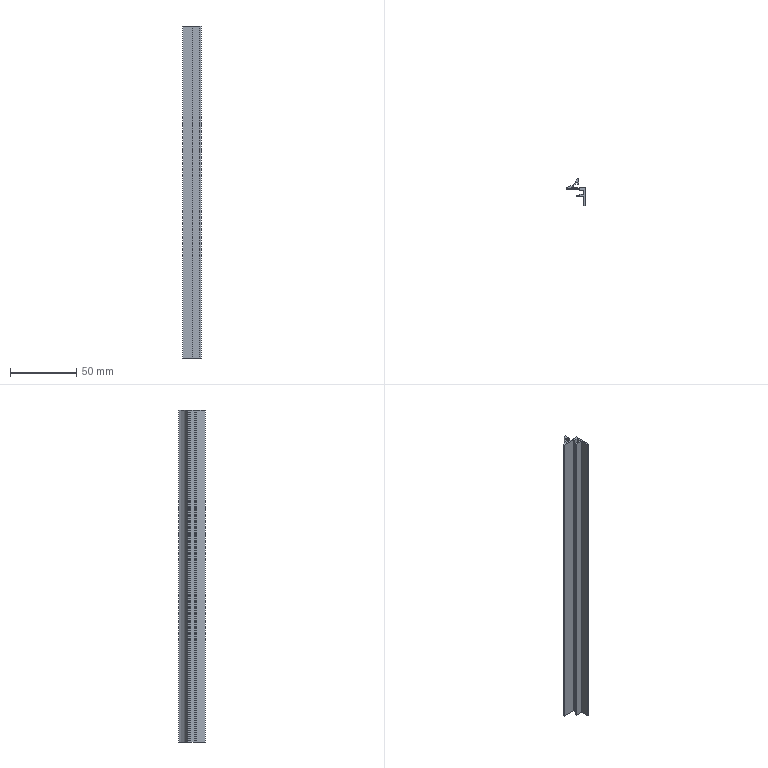Part | SolidWorks | features MoveFace 2, BaseBody 1, ICE 1 | 1 solid | 27 faces | box 14 x 20.3 x 251 mm | volume 12780 mm3 | plane 20 | cylinder 7 | commonest cylinder face diameters 0.387 x2 0.8 x2 0.4 x1 20 x1 22 x1
STEP:
#1=CARTESIAN_POINT('',(-5.304,-0.625,-289.));
#2=VERTEX_POINT('',#1);
#3=CARTESIAN_POINT('',(-5.449,-0.8125,-289.));
#4=VERTEX_POINT('',#3);
#5=CARTESIAN_POINT('',(-5.255,-0.8125,-289.));
#6=DIRECTION('',(0.,0.,1.));
#7=DIRECTION('',(-1.,0.,0.));
#8=AXIS2_PLACEMENT_3D('',#5,#6,#7);
#9=CIRCLE('',#8,0.1937);
#10=EDGE_CURVE('',#2,#4,#9,.T.);
#11=ORIENTED_EDGE('',*,*,#10,.T.);
#12=CARTESIAN_POINT('',(-5.449,-0.8125,-540.));
#13=VERTEX_POINT('',#12);
#14=CARTESIAN_POINT('',(-5.449,-0.8125,230.));
#15=DIRECTION('',(0.,0.,-1.));
#16=VECTOR('',#15,1000.);
#17=LINE('',#14,#16);
#18=EDGE_CURVE('',#4,#13,#17,.T.);
#19=ORIENTED_EDGE('',*,*,#18,.T.);
#20=CARTESIAN_POINT('',(-5.304,-0.625,-540.));
#21=VERTEX_POINT('',#20);
#22=CARTESIAN_POINT('',(-5.255,-0.8125,-540.));
#23=DIRECTION('',(0.,0.,-1.));
#24=DIRECTION('',(1.,0.,0.));
#25=AXIS2_PLACEMENT_3D('',#22,#23,#24);
#26=CIRCLE('',#25,0.1937);
#27=EDGE_CURVE('',#13,#21,#26,.T.);
#28=ORIENTED_EDGE('',*,*,#27,.T.);
#29=CARTESIAN_POINT('',(-5.304,-0.625,230.));
#30=DIRECTION('',(0.,0.,-1.));
#31=VECTOR('',#30,1000.);
#32=LINE('',#29,#31);
#33=EDGE_CURVE('',#2,#21,#32,.T.);
#34=ORIENTED_EDGE('',*,*,#33,.F.);
#35=EDGE_LOOP('',(#11,#19,#28,#34));
#36=FACE_OUTER_BOUND('',#35,.T.);
#37=CARTESIAN_POINT('',(-5.255,-0.8125,230.));
#38=DIRECTION('',(0.,0.,-1.));
#39=DIRECTION('',(-1.,0.,0.));
#40=AXIS2_PLACEMENT_3D('',#37,#38,#39);
#41=CYLINDRICAL_SURFACE('',#40,0.1937);
#42=ADVANCED_FACE('',(#36),#41,.F.);
#43=CARTESIAN_POINT('',(5.,-1.,-540.));
#44=VERTEX_POINT('',#43);
#45=CARTESIAN_POINT('',(5.,-14.3,-540.));
#46=VERTEX_POINT('',#45);
#47=CARTESIAN_POINT('',(5.,29.623,-540.));
#48=DIRECTION('',(0.,-1.,0.));
#49=VECTOR('',#48,1000.);
#50=LINE('',#47,#49);
#51=EDGE_CURVE('',#44,#46,#50,.T.);
#52=ORIENTED_EDGE('',*,*,#51,.F.);
#53=CARTESIAN_POINT('',(5.,-1.,-289.));
#54=VERTEX_POINT('',#53);
#55=CARTESIAN_POINT('',(5.,-1.,230.));
#56=DIRECTION('',(0.,0.,-1.));
#57=VECTOR('',#56,1000.);
#58=LINE('',#55,#57);
#59=EDGE_CURVE('',#54,#44,#58,.T.);
#60=ORIENTED_EDGE('',*,*,#59,.F.);
#61=CARTESIAN_POINT('',(5.,-14.3,-289.));
#62=VERTEX_POINT('',#61);
#63=CARTESIAN_POINT('',(5.,29.623,-289.));
#64=DIRECTION('',(0.,1.,0.));
#65=VECTOR('',#64,1000.);
#66=LINE('',#63,#65);
#67=EDGE_CURVE('',#62,#54,#66,.T.);
#68=ORIENTED_EDGE('',*,*,#67,.F.);
#69=CARTESIAN_POINT('',(5.,-14.3,230.));
#70=DIRECTION('',(0.,0.,1.));
#71=VECTOR('',#70,1000.);
#72=LINE('',#69,#71);
#73=EDGE_CURVE('',#46,#62,#72,.T.);
#74=ORIENTED_EDGE('',*,*,#73,.F.);
#75=EDGE_LOOP('',(#52,#60,#68,#74));
#76=FACE_OUTER_BOUND('',#75,.T.);
#77=CARTESIAN_POINT('',(5.,-14.3,230.));
#78=DIRECTION('',(-1.,0.,0.));
#79=DIRECTION('',(0.,0.,1.));
#80=AXIS2_PLACEMENT_3D('',#77,#78,#79);
#81=PLANE('',#80);
#82=ADVANCED_FACE('',(#76),#81,.F.);
#83=CARTESIAN_POINT('',(-9.,-2.,-540.));
#84=VERTEX_POINT('',#83);
#85=CARTESIAN_POINT('',(-9.,-2.,-289.));
#86=VERTEX_POINT('',#85);
#87=CARTESIAN_POINT('',(-9.,-2.,230.));
#88=DIRECTION('',(0.,0.,1.));
#89=VECTOR('',#88,1000.);
#90=LINE('',#87,#89);
#91=EDGE_CURVE('',#84,#86,#90,.T.);
#92=ORIENTED_EDGE('',*,*,#91,.F.);
#93=CARTESIAN_POINT('',(0.9,-2.,-540.));
#94=VERTEX_POINT('',#93);
#95=CARTESIAN_POINT('',(5.,-2.,-540.));
#96=DIRECTION('',(-1.,0.,0.));
#97=VECTOR('',#96,1000.);
#98=LINE('',#95,#97);
#99=EDGE_CURVE('',#94,#84,#98,.T.);
#100=ORIENTED_EDGE('',*,*,#99,.F.);
#101=CARTESIAN_POINT('',(0.9,-2.,-289.));
#102=VERTEX_POINT('',#101);
#103=CARTESIAN_POINT('',(0.9,-2.,230.));
#104=DIRECTION('',(0.,0.,-1.));
#105=VECTOR('',#104,1000.);
#106=LINE('',#103,#105);
#107=EDGE_CURVE('',#102,#94,#106,.T.);
#108=ORIENTED_EDGE('',*,*,#107,.F.);
#109=CARTESIAN_POINT('',(5.,-2.,-289.));
#110=DIRECTION('',(1.,0.,0.));
#111=VECTOR('',#110,1000.);
#112=LINE('',#109,#111);
#113=EDGE_CURVE('',#86,#102,#112,.T.);
#114=ORIENTED_EDGE('',*,*,#113,.F.);
#115=EDGE_LOOP('',(#92,#100,#108,#114));
#116=FACE_OUTER_BOUND('',#115,.T.);
#117=CARTESIAN_POINT('',(-9.,-2.,230.));
#118=DIRECTION('',(0.,1.,0.));
#119=DIRECTION('',(0.,0.,1.));
#120=AXIS2_PLACEMENT_3D('',#117,#118,#119);
#121=PLANE('',#120);
#122=ADVANCED_FACE('',(#116),#121,.F.);
#123=CARTESIAN_POINT('',(4.,-6.,-289.));
#124=VERTEX_POINT('',#123);
#125=CARTESIAN_POINT('',(4.,-3.,-289.));
#126=VERTEX_POINT('',#125);
#127=CARTESIAN_POINT('',(4.,-3.,-289.));
#128=DIRECTION('',(0.,1.,0.));
#129=VECTOR('',#128,1000.);
#130=LINE('',#127,#129);
#131=EDGE_CURVE('',#124,#126,#130,.T.);
#132=ORIENTED_EDGE('',*,*,#131,.F.);
#133=CARTESIAN_POINT('',(1.,-6.,-289.));
#134=VERTEX_POINT('',#133);
#135=CARTESIAN_POINT('',(4.,-6.,-289.));
#136=DIRECTION('',(1.,0.,0.));
#137=VECTOR('',#136,1000.);
#138=LINE('',#135,#137);
#139=EDGE_CURVE('',#134,#124,#138,.T.);
#140=ORIENTED_EDGE('',*,*,#139,.F.);
#141=CARTESIAN_POINT('',(1.,-6.7,-289.));
#142=VERTEX_POINT('',#141);
#143=CARTESIAN_POINT('',(1.,29.623,-289.));
#144=DIRECTION('',(0.,-1.,0.));
#145=VECTOR('',#144,1000.);
#146=LINE('',#143,#145);
#147=EDGE_CURVE('',#134,#142,#146,.T.);
#148=ORIENTED_EDGE('',*,*,#147,.T.);
#149=CARTESIAN_POINT('',(-1.7,-6.7,-289.));
#150=VERTEX_POINT('',#149);
#151=CARTESIAN_POINT('',(1.,-6.7,-289.));
#152=DIRECTION('',(1.,0.,0.));
#153=VECTOR('',#152,1000.);
#154=LINE('',#151,#153);
#155=EDGE_CURVE('',#150,#142,#154,.T.);
#156=ORIENTED_EDGE('',*,*,#155,.F.);
#157=CARTESIAN_POINT('',(-1.7,-7.7,-289.));
#158=VERTEX_POINT('',#157);
#159=CARTESIAN_POINT('',(-1.7,29.623,-289.));
#160=DIRECTION('',(0.,-1.,0.));
#161=VECTOR('',#160,1000.);
#162=LINE('',#159,#161);
#163=EDGE_CURVE('',#150,#158,#162,.T.);
#164=ORIENTED_EDGE('',*,*,#163,.T.);
#165=CARTESIAN_POINT('',(4.,-7.7,-289.));
#166=VERTEX_POINT('',#165);
#167=CARTESIAN_POINT('',(-1.7,-7.7,-289.));
#168=DIRECTION('',(-1.,0.,0.));
#169=VECTOR('',#168,1000.);
#170=LINE('',#167,#169);
#171=EDGE_CURVE('',#166,#158,#170,.T.);
#172=ORIENTED_EDGE('',*,*,#171,.F.);
#173=CARTESIAN_POINT('',(4.,-14.3,-289.));
#174=VERTEX_POINT('',#173);
#175=CARTESIAN_POINT('',(4.,-7.7,-289.));
#176=DIRECTION('',(0.,1.,0.));
#177=VECTOR('',#176,1000.);
#178=LINE('',#175,#177);
#179=EDGE_CURVE('',#174,#166,#178,.T.);
#180=ORIENTED_EDGE('',*,*,#179,.F.);
#181=CARTESIAN_POINT('',(4.,-14.3,-289.));
#182=DIRECTION('',(-1.,0.,0.));
#183=VECTOR('',#182,1000.);
#184=LINE('',#181,#183);
#185=EDGE_CURVE('',#62,#174,#184,.T.);
#186=ORIENTED_EDGE('',*,*,#185,.F.);
#187=ORIENTED_EDGE('',*,*,#67,.T.);
#188=CARTESIAN_POINT('',(-5.207,-1.,-289.));
#189=VERTEX_POINT('',#188);
#190=CARTESIAN_POINT('',(5.,-1.,-289.));
#191=DIRECTION('',(1.,0.,0.));
#192=VECTOR('',#191,1000.);
#193=LINE('',#190,#192);
#194=EDGE_CURVE('',#189,#54,#193,.T.);
#195=ORIENTED_EDGE('',*,*,#194,.F.);
#196=CARTESIAN_POINT('',(-5.255,-0.8125,-289.));
#197=DIRECTION('',(0.,0.,1.));
#198=DIRECTION('',(-1.,0.,0.));
#199=AXIS2_PLACEMENT_3D('',#196,#197,#198);
#200=CIRCLE('',#199,0.1937);
#201=EDGE_CURVE('',#4,#189,#200,.T.);
#202=ORIENTED_EDGE('',*,*,#201,.F.);
#203=ORIENTED_EDGE('',*,*,#10,.F.);
#204=CARTESIAN_POINT('',(-1.368,3.063,-289.));
#205=VERTEX_POINT('',#204);
#206=CARTESIAN_POINT('',(-10.628,9.,-289.));
#207=DIRECTION('',(0.,0.,1.));
#208=DIRECTION('',(-1.,0.,0.));
#209=AXIS2_PLACEMENT_3D('',#206,#207,#208);
#210=CIRCLE('',#209,11.);
#211=EDGE_CURVE('',#2,#205,#210,.T.);
#212=ORIENTED_EDGE('',*,*,#211,.T.);
#213=CARTESIAN_POINT('',(-1.,2.955,-289.));
#214=VERTEX_POINT('',#213);
#215=CARTESIAN_POINT('',(-1.2,2.955,-289.));
#216=DIRECTION('',(0.,0.,1.));
#217=DIRECTION('',(-1.,0.,0.));
#218=AXIS2_PLACEMENT_3D('',#215,#216,#217);
#219=CIRCLE('',#218,0.2);
#220=EDGE_CURVE('',#214,#205,#219,.T.);
#221=ORIENTED_EDGE('',*,*,#220,.F.);
#222=CARTESIAN_POINT('',(-1.,1.5,-289.));
#223=VERTEX_POINT('',#222);
#224=CARTESIAN_POINT('',(-1.,2.955,-289.));
#225=DIRECTION('',(0.,1.,0.));
#226=VECTOR('',#225,1000.);
#227=LINE('',#224,#226);
#228=EDGE_CURVE('',#223,#214,#227,.T.);
#229=ORIENTED_EDGE('',*,*,#228,.F.);
#230=CARTESIAN_POINT('',(0.,1.5,-289.));
#231=VERTEX_POINT('',#230);
#232=CARTESIAN_POINT('',(-1.,1.5,-289.));
#233=DIRECTION('',(-1.,0.,0.));
#234=VECTOR('',#233,1000.);
#235=LINE('',#232,#234);
#236=EDGE_CURVE('',#231,#223,#235,.T.);
#237=ORIENTED_EDGE('',*,*,#236,.F.);
#238=CARTESIAN_POINT('',(0.,6.,-289.));
#239=VERTEX_POINT('',#238);
#240=CARTESIAN_POINT('',(0.,1.5,-289.));
#241=DIRECTION('',(0.,-1.,0.));
#242=VECTOR('',#241,1000.);
#243=LINE('',#240,#242);
#244=EDGE_CURVE('',#239,#231,#243,.T.);
#245=ORIENTED_EDGE('',*,*,#244,.F.);
#246=CARTESIAN_POINT('',(-0.8,6.,-289.));
#247=VERTEX_POINT('',#246);
#248=CARTESIAN_POINT('',(0.,6.,-289.));
#249=DIRECTION('',(1.,0.,0.));
#250=VECTOR('',#249,1000.);
#251=LINE('',#248,#250);
#252=EDGE_CURVE('',#247,#239,#251,.T.);
#253=ORIENTED_EDGE('',*,*,#252,.F.);
#254=CARTESIAN_POINT('',(-1.178,5.731,-289.));
#255=VERTEX_POINT('',#254);
#256=CARTESIAN_POINT('',(-0.8,5.6,-289.));
#257=DIRECTION('',(0.,0.,1.));
#258=DIRECTION('',(-1.,0.,0.));
#259=AXIS2_PLACEMENT_3D('',#256,#257,#258);
#260=CIRCLE('',#259,0.4);
#261=EDGE_CURVE('',#247,#255,#260,.T.);
#262=ORIENTED_EDGE('',*,*,#261,.T.);
#263=CARTESIAN_POINT('',(-8.678,-0.8077,-289.));
#264=VERTEX_POINT('',#263);
#265=CARTESIAN_POINT('',(-10.628,9.,-289.));
#266=DIRECTION('',(0.,0.,1.));
#267=DIRECTION('',(-1.,0.,0.));
#268=AXIS2_PLACEMENT_3D('',#265,#266,#267);
#269=CIRCLE('',#268,10.);
#270=EDGE_CURVE('',#264,#255,#269,.T.);
#271=ORIENTED_EDGE('',*,*,#270,.F.);
#272=CARTESIAN_POINT('',(-9.,-1.2,-289.));
#273=VERTEX_POINT('',#272);
#274=CARTESIAN_POINT('',(-8.6,-1.2,-289.));
#275=DIRECTION('',(0.,0.,1.));
#276=DIRECTION('',(-1.,0.,0.));
#277=AXIS2_PLACEMENT_3D('',#274,#275,#276);
#278=CIRCLE('',#277,0.4);
#279=EDGE_CURVE('',#264,#273,#278,.T.);
#280=ORIENTED_EDGE('',*,*,#279,.T.);
#281=CARTESIAN_POINT('',(-9.,29.623,-289.));
#282=DIRECTION('',(0.,-1.,0.));
#283=VECTOR('',#282,1000.);
#284=LINE('',#281,#283);
#285=EDGE_CURVE('',#273,#86,#284,.T.);
#286=ORIENTED_EDGE('',*,*,#285,.T.);
#287=ORIENTED_EDGE('',*,*,#113,.T.);
#288=CARTESIAN_POINT('',(0.9,-3.,-289.));
#289=VERTEX_POINT('',#288);
#290=CARTESIAN_POINT('',(0.9,-2.,-289.));
#291=DIRECTION('',(0.,1.,0.));
#292=VECTOR('',#291,1000.);
#293=LINE('',#290,#292);
#294=EDGE_CURVE('',#289,#102,#293,.T.);
#295=ORIENTED_EDGE('',*,*,#294,.F.);
#296=CARTESIAN_POINT('',(0.9,-3.,-289.));
#297=DIRECTION('',(-1.,0.,0.));
#298=VECTOR('',#297,1000.);
#299=LINE('',#296,#298);
#300=EDGE_CURVE('',#126,#289,#299,.T.);
#301=ORIENTED_EDGE('',*,*,#300,.F.);
#302=EDGE_LOOP('',(#132,#140,#148,#156,#164,#172,#180,#186,#187,#195,#202,#203,#212,#221,#229,#237,#245,#253,#262,#271,#280,#286,#287,#295,#301));
#303=FACE_OUTER_BOUND('',#302,.T.);
#304=CARTESIAN_POINT('',(5.,29.623,-289.));
#305=DIRECTION('',(0.,0.,-1.));
#306=DIRECTION('',(-1.,0.,0.));
#307=AXIS2_PLACEMENT_3D('',#304,#305,#306);
#308=PLANE('',#307);
#309=ADVANCED_FACE('',(#303),#308,.F.);
#310=ORIENTED_EDGE('',*,*,#185,.T.);
#311=CARTESIAN_POINT('',(4.,-14.3,-540.));
#312=VERTEX_POINT('',#311);
#313=CARTESIAN_POINT('',(4.,-14.3,230.));
#314=DIRECTION('',(0.,0.,1.));
#315=VECTOR('',#314,1000.);
#316=LINE('',#313,#315);
#317=EDGE_CURVE('',#312,#174,#316,.T.);
#318=ORIENTED_EDGE('',*,*,#317,.F.);
#319=CARTESIAN_POINT('',(5.,-14.3,-540.));
#320=DIRECTION('',(-1.,0.,0.));
#321=VECTOR('',#320,1000.);
#322=LINE('',#319,#321);
#323=EDGE_CURVE('',#46,#312,#322,.T.);
#324=ORIENTED_EDGE('',*,*,#323,.F.);
#325=ORIENTED_EDGE('',*,*,#73,.T.);
#326=EDGE_LOOP('',(#310,#318,#324,#325));
#327=FACE_OUTER_BOUND('',#326,.T.);
#328=CARTESIAN_POINT('',(4.,-14.3,230.));
#329=DIRECTION('',(0.,1.,0.));
#330=DIRECTION('',(0.,0.,1.));
#331=AXIS2_PLACEMENT_3D('',#328,#329,#330);
#332=PLANE('',#331);
#333=ADVANCED_FACE('',(#327),#332,.F.);
#334=ORIENTED_EDGE('',*,*,#51,.T.);
#335=ORIENTED_EDGE('',*,*,#323,.T.);
#336=CARTESIAN_POINT('',(4.,-7.7,-540.));
#337=VERTEX_POINT('',#336);
#338=CARTESIAN_POINT('',(4.,-7.7,-540.));
#339=DIRECTION('',(0.,-1.,0.));
#340=VECTOR('',#339,1000.);
#341=LINE('',#338,#340);
#342=EDGE_CURVE('',#337,#312,#341,.T.);
#343=ORIENTED_EDGE('',*,*,#342,.F.);
#344=CARTESIAN_POINT('',(-1.7,-7.7,-540.));
#345=VERTEX_POINT('',#344);
#346=CARTESIAN_POINT('',(-1.7,-7.7,-540.));
#347=DIRECTION('',(1.,0.,0.));
#348=VECTOR('',#347,1000.);
#349=LINE('',#346,#348);
#350=EDGE_CURVE('',#345,#337,#349,.T.);
#351=ORIENTED_EDGE('',*,*,#350,.F.);
#352=CARTESIAN_POINT('',(-1.7,-6.7,-540.));
#353=VERTEX_POINT('',#352);
#354=CARTESIAN_POINT('',(-1.7,29.623,-540.));
#355=DIRECTION('',(0.,1.,0.));
#356=VECTOR('',#355,1000.);
#357=LINE('',#354,#356);
#358=EDGE_CURVE('',#345,#353,#357,.T.);
#359=ORIENTED_EDGE('',*,*,#358,.T.);
#360=CARTESIAN_POINT('',(1.,-6.7,-540.));
#361=VERTEX_POINT('',#360);
#362=CARTESIAN_POINT('',(1.,-6.7,-540.));
#363=DIRECTION('',(-1.,0.,0.));
#364=VECTOR('',#363,1000.);
#365=LINE('',#362,#364);
#366=EDGE_CURVE('',#361,#353,#365,.T.);
#367=ORIENTED_EDGE('',*,*,#366,.F.);
#368=CARTESIAN_POINT('',(1.,-6.,-540.));
#369=VERTEX_POINT('',#368);
#370=CARTESIAN_POINT('',(1.,29.623,-540.));
#371=DIRECTION('',(0.,1.,0.));
#372=VECTOR('',#371,1000.);
#373=LINE('',#370,#372);
#374=EDGE_CURVE('',#361,#369,#373,.T.);
#375=ORIENTED_EDGE('',*,*,#374,.T.);
#376=CARTESIAN_POINT('',(4.,-6.,-540.));
#377=VERTEX_POINT('',#376);
#378=CARTESIAN_POINT('',(4.,-6.,-540.));
#379=DIRECTION('',(-1.,0.,0.));
#380=VECTOR('',#379,1000.);
#381=LINE('',#378,#380);
#382=EDGE_CURVE('',#377,#369,#381,.T.);
#383=ORIENTED_EDGE('',*,*,#382,.F.);
#384=CARTESIAN_POINT('',(4.,-3.,-540.));
#385=VERTEX_POINT('',#384);
#386=CARTESIAN_POINT('',(4.,-3.,-540.));
#387=DIRECTION('',(0.,-1.,0.));
#388=VECTOR('',#387,1000.);
#389=LINE('',#386,#388);
#390=EDGE_CURVE('',#385,#377,#389,.T.);
#391=ORIENTED_EDGE('',*,*,#390,.F.);
#392=CARTESIAN_POINT('',(0.9,-3.,-540.));
#393=VERTEX_POINT('',#392);
#394=CARTESIAN_POINT('',(0.9,-3.,-540.));
#395=DIRECTION('',(1.,0.,0.));
#396=VECTOR('',#395,1000.);
#397=LINE('',#394,#396);
#398=EDGE_CURVE('',#393,#385,#397,.T.);
#399=ORIENTED_EDGE('',*,*,#398,.F.);
#400=CARTESIAN_POINT('',(0.9,-2.,-540.));
#401=DIRECTION('',(0.,-1.,0.));
#402=VECTOR('',#401,1000.);
#403=LINE('',#400,#402);
#404=EDGE_CURVE('',#94,#393,#403,.T.);
#405=ORIENTED_EDGE('',*,*,#404,.F.);
#406=ORIENTED_EDGE('',*,*,#99,.T.);
#407=CARTESIAN_POINT('',(-9.,-1.2,-540.));
#408=VERTEX_POINT('',#407);
#409=CARTESIAN_POINT('',(-9.,-1.2,-540.));
#410=DIRECTION('',(0.,-1.,0.));
#411=VECTOR('',#410,1000.);
#412=LINE('',#409,#411);
#413=EDGE_CURVE('',#408,#84,#412,.T.);
#414=ORIENTED_EDGE('',*,*,#413,.F.);
#415=CARTESIAN_POINT('',(-8.678,-0.8077,-540.));
#416=VERTEX_POINT('',#415);
#417=CARTESIAN_POINT('',(-8.6,-1.2,-540.));
#418=DIRECTION('',(0.,0.,-1.));
#419=DIRECTION('',(1.,0.,0.));
#420=AXIS2_PLACEMENT_3D('',#417,#418,#419);
#421=CIRCLE('',#420,0.4);
#422=EDGE_CURVE('',#408,#416,#421,.T.);
#423=ORIENTED_EDGE('',*,*,#422,.T.);
#424=CARTESIAN_POINT('',(-1.178,5.731,-540.));
#425=VERTEX_POINT('',#424);
#426=CARTESIAN_POINT('',(-10.628,9.,-540.));
#427=DIRECTION('',(0.,0.,-1.));
#428=DIRECTION('',(1.,0.,0.));
#429=AXIS2_PLACEMENT_3D('',#426,#427,#428);
#430=CIRCLE('',#429,10.);
#431=EDGE_CURVE('',#425,#416,#430,.T.);
#432=ORIENTED_EDGE('',*,*,#431,.F.);
#433=CARTESIAN_POINT('',(-0.8,6.,-540.));
#434=VERTEX_POINT('',#433);
#435=CARTESIAN_POINT('',(-0.8,5.6,-540.));
#436=DIRECTION('',(0.,0.,-1.));
#437=DIRECTION('',(1.,0.,0.));
#438=AXIS2_PLACEMENT_3D('',#435,#436,#437);
#439=CIRCLE('',#438,0.4);
#440=EDGE_CURVE('',#425,#434,#439,.T.);
#441=ORIENTED_EDGE('',*,*,#440,.T.);
#442=CARTESIAN_POINT('',(0.,6.,-540.));
#443=VERTEX_POINT('',#442);
#444=CARTESIAN_POINT('',(0.,6.,-540.));
#445=DIRECTION('',(-1.,0.,0.));
#446=VECTOR('',#445,1000.);
#447=LINE('',#444,#446);
#448=EDGE_CURVE('',#443,#434,#447,.T.);
#449=ORIENTED_EDGE('',*,*,#448,.F.);
#450=CARTESIAN_POINT('',(0.,1.5,-540.));
#451=VERTEX_POINT('',#450);
#452=CARTESIAN_POINT('',(0.,1.5,-540.));
#453=DIRECTION('',(0.,1.,0.));
#454=VECTOR('',#453,1000.);
#455=LINE('',#452,#454);
#456=EDGE_CURVE('',#451,#443,#455,.T.);
#457=ORIENTED_EDGE('',*,*,#456,.F.);
#458=CARTESIAN_POINT('',(-1.,1.5,-540.));
#459=VERTEX_POINT('',#458);
#460=CARTESIAN_POINT('',(-1.,1.5,-540.));
#461=DIRECTION('',(1.,0.,0.));
#462=VECTOR('',#461,1000.);
#463=LINE('',#460,#462);
#464=EDGE_CURVE('',#459,#451,#463,.T.);
#465=ORIENTED_EDGE('',*,*,#464,.F.);
#466=CARTESIAN_POINT('',(-1.,2.955,-540.));
#467=VERTEX_POINT('',#466);
#468=CARTESIAN_POINT('',(-1.,2.955,-540.));
#469=DIRECTION('',(0.,-1.,0.));
#470=VECTOR('',#469,1000.);
#471=LINE('',#468,#470);
#472=EDGE_CURVE('',#467,#459,#471,.T.);
#473=ORIENTED_EDGE('',*,*,#472,.F.);
#474=CARTESIAN_POINT('',(-1.368,3.063,-540.));
#475=VERTEX_POINT('',#474);
#476=CARTESIAN_POINT('',(-1.2,2.955,-540.));
#477=DIRECTION('',(0.,0.,-1.));
#478=DIRECTION('',(1.,0.,0.));
#479=AXIS2_PLACEMENT_3D('',#476,#477,#478);
#480=CIRCLE('',#479,0.2);
#481=EDGE_CURVE('',#475,#467,#480,.T.);
#482=ORIENTED_EDGE('',*,*,#481,.F.);
#483=CARTESIAN_POINT('',(-10.628,9.,-540.));
#484=DIRECTION('',(0.,0.,-1.));
#485=DIRECTION('',(1.,0.,0.));
#486=AXIS2_PLACEMENT_3D('',#483,#484,#485);
#487=CIRCLE('',#486,11.);
#488=EDGE_CURVE('',#475,#21,#487,.T.);
#489=ORIENTED_EDGE('',*,*,#488,.T.);
#490=ORIENTED_EDGE('',*,*,#27,.F.);
#491=CARTESIAN_POINT('',(-5.207,-1.,-540.));
#492=VERTEX_POINT('',#491);
#493=CARTESIAN_POINT('',(-5.255,-0.8125,-540.));
#494=DIRECTION('',(0.,0.,-1.));
#495=DIRECTION('',(1.,0.,0.));
#496=AXIS2_PLACEMENT_3D('',#493,#494,#495);
#497=CIRCLE('',#496,0.1937);
#498=EDGE_CURVE('',#492,#13,#497,.T.);
#499=ORIENTED_EDGE('',*,*,#498,.F.);
#500=CARTESIAN_POINT('',(5.,-1.,-540.));
#501=DIRECTION('',(-1.,0.,0.));
#502=VECTOR('',#501,1000.);
#503=LINE('',#500,#502);
#504=EDGE_CURVE('',#44,#492,#503,.T.);
#505=ORIENTED_EDGE('',*,*,#504,.F.);
#506=EDGE_LOOP('',(#334,#335,#343,#351,#359,#367,#375,#383,#391,#399,#405,#406,#414,#423,#432,#441,#449,#457,#465,#473,#482,#489,#490,#499,#505));
#507=FACE_OUTER_BOUND('',#506,.T.);
#508=CARTESIAN_POINT('',(5.,29.623,-540.));
#509=DIRECTION('',(0.,0.,1.));
#510=DIRECTION('',(1.,0.,0.));
#511=AXIS2_PLACEMENT_3D('',#508,#509,#510);
#512=PLANE('',#511);
#513=ADVANCED_FACE('',(#507),#512,.F.);
#514=ORIENTED_EDGE('',*,*,#59,.T.);
#515=ORIENTED_EDGE('',*,*,#504,.T.);
#516=CARTESIAN_POINT('',(-5.207,-1.,230.));
#517=DIRECTION('',(0.,0.,-1.));
#518=VECTOR('',#517,1000.);
#519=LINE('',#516,#518);
#520=EDGE_CURVE('',#189,#492,#519,.T.);
#521=ORIENTED_EDGE('',*,*,#520,.F.);
#522=ORIENTED_EDGE('',*,*,#194,.T.);
#523=EDGE_LOOP('',(#514,#515,#521,#522));
#524=FACE_OUTER_BOUND('',#523,.T.);
#525=CARTESIAN_POINT('',(5.,-1.,230.));
#526=DIRECTION('',(0.,-1.,0.));
#527=DIRECTION('',(0.,0.,-1.));
#528=AXIS2_PLACEMENT_3D('',#525,#526,#527);
#529=PLANE('',#528);
#530=ADVANCED_FACE('',(#524),#529,.F.);
#531=CARTESIAN_POINT('',(-9.,-1.2,230.));
#532=DIRECTION('',(0.,0.,1.));
#533=VECTOR('',#532,1000.);
#534=LINE('',#531,#533);
#535=EDGE_CURVE('',#408,#273,#534,.T.);
#536=ORIENTED_EDGE('',*,*,#535,.F.);
#537=ORIENTED_EDGE('',*,*,#413,.T.);
#538=ORIENTED_EDGE('',*,*,#91,.T.);
#539=ORIENTED_EDGE('',*,*,#285,.F.);
#540=EDGE_LOOP('',(#536,#537,#538,#539));
#541=FACE_OUTER_BOUND('',#540,.T.);
#542=CARTESIAN_POINT('',(-9.,-1.2,230.));
#543=DIRECTION('',(1.,0.,0.));
#544=DIRECTION('',(0.,0.,-1.));
#545=AXIS2_PLACEMENT_3D('',#542,#543,#544);
#546=PLANE('',#545);
#547=ADVANCED_FACE('',(#541),#546,.F.);
#548=ORIENTED_EDGE('',*,*,#294,.T.);
#549=ORIENTED_EDGE('',*,*,#107,.T.);
#550=ORIENTED_EDGE('',*,*,#404,.T.);
#551=CARTESIAN_POINT('',(0.9,-3.,230.));
#552=DIRECTION('',(0.,0.,-1.));
#553=VECTOR('',#552,1000.);
#554=LINE('',#551,#553);
#555=EDGE_CURVE('',#289,#393,#554,.T.);
#556=ORIENTED_EDGE('',*,*,#555,.F.);
#557=EDGE_LOOP('',(#548,#549,#550,#556));
#558=FACE_OUTER_BOUND('',#557,.T.);
#559=CARTESIAN_POINT('',(0.9,-2.,230.));
#560=DIRECTION('',(1.,0.,0.));
#561=DIRECTION('',(0.,0.,-1.));
#562=AXIS2_PLACEMENT_3D('',#559,#560,#561);
#563=PLANE('',#562);
#564=ADVANCED_FACE('',(#558),#563,.F.);
#565=ORIENTED_EDGE('',*,*,#300,.T.);
#566=ORIENTED_EDGE('',*,*,#555,.T.);
#567=ORIENTED_EDGE('',*,*,#398,.T.);
#568=CARTESIAN_POINT('',(4.,-3.,230.));
#569=DIRECTION('',(0.,0.,-1.));
#570=VECTOR('',#569,1000.);
#571=LINE('',#568,#570);
#572=EDGE_CURVE('',#126,#385,#571,.T.);
#573=ORIENTED_EDGE('',*,*,#572,.F.);
#574=EDGE_LOOP('',(#565,#566,#567,#573));
#575=FACE_OUTER_BOUND('',#574,.T.);
#576=CARTESIAN_POINT('',(0.9,-3.,230.));
#577=DIRECTION('',(0.,1.,0.));
#578=DIRECTION('',(0.,0.,1.));
#579=AXIS2_PLACEMENT_3D('',#576,#577,#578);
#580=PLANE('',#579);
#581=ADVANCED_FACE('',(#575),#580,.F.);
#582=ORIENTED_EDGE('',*,*,#131,.T.);
#583=ORIENTED_EDGE('',*,*,#572,.T.);
#584=ORIENTED_EDGE('',*,*,#390,.T.);
#585=CARTESIAN_POINT('',(4.,-6.,230.));
#586=DIRECTION('',(0.,0.,-1.));
#587=VECTOR('',#586,1000.);
#588=LINE('',#585,#587);
#589=EDGE_CURVE('',#124,#377,#588,.T.);
#590=ORIENTED_EDGE('',*,*,#589,.F.);
#591=EDGE_LOOP('',(#582,#583,#584,#590));
#592=FACE_OUTER_BOUND('',#591,.T.);
#593=CARTESIAN_POINT('',(4.,-3.,230.));
#594=DIRECTION('',(1.,0.,0.));
#595=DIRECTION('',(0.,0.,-1.));
#596=AXIS2_PLACEMENT_3D('',#593,#594,#595);
#597=PLANE('',#596);
#598=ADVANCED_FACE('',(#592),#597,.F.);
#599=ORIENTED_EDGE('',*,*,#139,.T.);
#600=ORIENTED_EDGE('',*,*,#589,.T.);
#601=ORIENTED_EDGE('',*,*,#382,.T.);
#602=CARTESIAN_POINT('',(1.,-6.,230.));
#603=DIRECTION('',(0.,0.,-1.));
#604=VECTOR('',#603,1000.);
#605=LINE('',#602,#604);
#606=EDGE_CURVE('',#134,#369,#605,.T.);
#607=ORIENTED_EDGE('',*,*,#606,.F.);
#608=EDGE_LOOP('',(#599,#600,#601,#607));
#609=FACE_OUTER_BOUND('',#608,.T.);
#610=CARTESIAN_POINT('',(4.,-6.,230.));
#611=DIRECTION('',(0.,-1.,0.));
#612=DIRECTION('',(0.,0.,-1.));
#613=AXIS2_PLACEMENT_3D('',#610,#611,#612);
#614=PLANE('',#613);
#615=ADVANCED_FACE('',(#609),#614,.F.);
#616=ORIENTED_EDGE('',*,*,#155,.T.);
#617=CARTESIAN_POINT('',(1.,-6.7,230.));
#618=DIRECTION('',(0.,0.,1.));
#619=VECTOR('',#618,1000.);
#620=LINE('',#617,#619);
#621=EDGE_CURVE('',#361,#142,#620,.T.);
#622=ORIENTED_EDGE('',*,*,#621,.F.);
#623=ORIENTED_EDGE('',*,*,#366,.T.);
#624=CARTESIAN_POINT('',(-1.7,-6.7,230.));
#625=DIRECTION('',(0.,0.,-1.));
#626=VECTOR('',#625,1000.);
#627=LINE('',#624,#626);
#628=EDGE_CURVE('',#150,#353,#627,.T.);
#629=ORIENTED_EDGE('',*,*,#628,.F.);
#630=EDGE_LOOP('',(#616,#622,#623,#629));
#631=FACE_OUTER_BOUND('',#630,.T.);
#632=CARTESIAN_POINT('',(1.,-6.7,230.));
#633=DIRECTION('',(0.,-1.,0.));
#634=DIRECTION('',(0.,0.,-1.));
#635=AXIS2_PLACEMENT_3D('',#632,#633,#634);
#636=PLANE('',#635);
#637=ADVANCED_FACE('',(#631),#636,.F.);
#638=ORIENTED_EDGE('',*,*,#171,.T.);
#639=CARTESIAN_POINT('',(-1.7,-7.7,230.));
#640=DIRECTION('',(0.,0.,1.));
#641=VECTOR('',#640,1000.);
#642=LINE('',#639,#641);
#643=EDGE_CURVE('',#345,#158,#642,.T.);
#644=ORIENTED_EDGE('',*,*,#643,.F.);
#645=ORIENTED_EDGE('',*,*,#350,.T.);
#646=CARTESIAN_POINT('',(4.,-7.7,230.));
#647=DIRECTION('',(0.,0.,-1.));
#648=VECTOR('',#647,1000.);
#649=LINE('',#646,#648);
#650=EDGE_CURVE('',#166,#337,#649,.T.);
#651=ORIENTED_EDGE('',*,*,#650,.F.);
#652=EDGE_LOOP('',(#638,#644,#645,#651));
#653=FACE_OUTER_BOUND('',#652,.T.);
#654=CARTESIAN_POINT('',(-1.7,-7.7,230.));
#655=DIRECTION('',(0.,1.,0.));
#656=DIRECTION('',(0.,0.,1.));
#657=AXIS2_PLACEMENT_3D('',#654,#655,#656);
#658=PLANE('',#657);
#659=ADVANCED_FACE('',(#653),#658,.F.);
#660=ORIENTED_EDGE('',*,*,#179,.T.);
#661=ORIENTED_EDGE('',*,*,#650,.T.);
#662=ORIENTED_EDGE('',*,*,#342,.T.);
#663=ORIENTED_EDGE('',*,*,#317,.T.);
#664=EDGE_LOOP('',(#660,#661,#662,#663));
#665=FACE_OUTER_BOUND('',#664,.T.);
#666=CARTESIAN_POINT('',(4.,-7.7,230.));
#667=DIRECTION('',(1.,0.,0.));
#668=DIRECTION('',(0.,0.,-1.));
#669=AXIS2_PLACEMENT_3D('',#666,#667,#668);
#670=PLANE('',#669);
#671=ADVANCED_FACE('',(#665),#670,.F.);
#672=ORIENTED_EDGE('',*,*,#18,.F.);
#673=ORIENTED_EDGE('',*,*,#201,.T.);
#674=ORIENTED_EDGE('',*,*,#520,.T.);
#675=ORIENTED_EDGE('',*,*,#498,.T.);
#676=EDGE_LOOP('',(#672,#673,#674,#675));
#677=FACE_OUTER_BOUND('',#676,.T.);
#678=CARTESIAN_POINT('',(-5.255,-0.8125,230.));
#679=DIRECTION('',(0.,0.,-1.));
#680=DIRECTION('',(-1.,0.,0.));
#681=AXIS2_PLACEMENT_3D('',#678,#679,#680);
#682=CYLINDRICAL_SURFACE('',#681,0.1937);
#683=ADVANCED_FACE('',(#677),#682,.F.);
#684=CARTESIAN_POINT('',(-1.,2.955,230.));
#685=DIRECTION('',(0.,0.,1.));
#686=VECTOR('',#685,1000.);
#687=LINE('',#684,#686);
#688=EDGE_CURVE('',#467,#214,#687,.T.);
#689=ORIENTED_EDGE('',*,*,#688,.F.);
#690=ORIENTED_EDGE('',*,*,#472,.T.);
#691=CARTESIAN_POINT('',(-1.,1.5,230.));
#692=DIRECTION('',(0.,0.,-1.));
#693=VECTOR('',#692,1000.);
#694=LINE('',#691,#693);
#695=EDGE_CURVE('',#223,#459,#694,.T.);
#696=ORIENTED_EDGE('',*,*,#695,.F.);
#697=ORIENTED_EDGE('',*,*,#228,.T.);
#698=EDGE_LOOP('',(#689,#690,#696,#697));
#699=FACE_OUTER_BOUND('',#698,.T.);
#700=CARTESIAN_POINT('',(-1.,2.955,230.));
#701=DIRECTION('',(1.,0.,0.));
#702=DIRECTION('',(0.,0.,-1.));
#703=AXIS2_PLACEMENT_3D('',#700,#701,#702);
#704=PLANE('',#703);
#705=ADVANCED_FACE('',(#699),#704,.F.);
#706=ORIENTED_EDGE('',*,*,#488,.F.);
#707=CARTESIAN_POINT('',(-1.368,3.063,230.));
#708=DIRECTION('',(0.,0.,1.));
#709=VECTOR('',#708,1000.);
#710=LINE('',#707,#709);
#711=EDGE_CURVE('',#475,#205,#710,.T.);
#712=ORIENTED_EDGE('',*,*,#711,.T.);
#713=ORIENTED_EDGE('',*,*,#211,.F.);
#714=ORIENTED_EDGE('',*,*,#33,.T.);
#715=EDGE_LOOP('',(#706,#712,#713,#714));
#716=FACE_OUTER_BOUND('',#715,.T.);
#717=CARTESIAN_POINT('',(-10.628,9.,230.));
#718=DIRECTION('',(0.,0.,-1.));
#719=DIRECTION('',(-1.,0.,0.));
#720=AXIS2_PLACEMENT_3D('',#717,#718,#719);
#721=CYLINDRICAL_SURFACE('',#720,11.);
#722=ADVANCED_FACE('',(#716),#721,.T.);
#723=CARTESIAN_POINT('',(-1.178,5.731,230.));
#724=DIRECTION('',(0.,0.,1.));
#725=VECTOR('',#724,1000.);
#726=LINE('',#723,#725);
#727=EDGE_CURVE('',#425,#255,#726,.T.);
#728=ORIENTED_EDGE('',*,*,#727,.F.);
#729=ORIENTED_EDGE('',*,*,#431,.T.);
#730=CARTESIAN_POINT('',(-8.678,-0.8077,230.));
#731=DIRECTION('',(0.,0.,-1.));
#732=VECTOR('',#731,1000.);
#733=LINE('',#730,#732);
#734=EDGE_CURVE('',#264,#416,#733,.T.);
#735=ORIENTED_EDGE('',*,*,#734,.F.);
#736=ORIENTED_EDGE('',*,*,#270,.T.);
#737=EDGE_LOOP('',(#728,#729,#735,#736));
#738=FACE_OUTER_BOUND('',#737,.T.);
#739=CARTESIAN_POINT('',(-10.628,9.,230.));
#740=DIRECTION('',(0.,0.,-1.));
#741=DIRECTION('',(-1.,0.,0.));
#742=AXIS2_PLACEMENT_3D('',#739,#740,#741);
#743=CYLINDRICAL_SURFACE('',#742,10.);
#744=ADVANCED_FACE('',(#738),#743,.F.);
#745=CARTESIAN_POINT('',(0.,1.5,230.));
#746=DIRECTION('',(0.,0.,1.));
#747=VECTOR('',#746,1000.);
#748=LINE('',#745,#747);
#749=EDGE_CURVE('',#451,#231,#748,.T.);
#750=ORIENTED_EDGE('',*,*,#749,.F.);
#751=ORIENTED_EDGE('',*,*,#456,.T.);
#752=CARTESIAN_POINT('',(0.,6.,230.));
#753=DIRECTION('',(0.,0.,-1.));
#754=VECTOR('',#753,1000.);
#755=LINE('',#752,#754);
#756=EDGE_CURVE('',#239,#443,#755,.T.);
#757=ORIENTED_EDGE('',*,*,#756,.F.);
#758=ORIENTED_EDGE('',*,*,#244,.T.);
#759=EDGE_LOOP('',(#750,#751,#757,#758));
#760=FACE_OUTER_BOUND('',#759,.T.);
#761=CARTESIAN_POINT('',(0.,1.5,230.));
#762=DIRECTION('',(-1.,0.,0.));
#763=DIRECTION('',(0.,0.,1.));
#764=AXIS2_PLACEMENT_3D('',#761,#762,#763);
#765=PLANE('',#764);
#766=ADVANCED_FACE('',(#760),#765,.F.);
#767=ORIENTED_EDGE('',*,*,#422,.F.);
#768=ORIENTED_EDGE('',*,*,#535,.T.);
#769=ORIENTED_EDGE('',*,*,#279,.F.);
#770=ORIENTED_EDGE('',*,*,#734,.T.);
#771=EDGE_LOOP('',(#767,#768,#769,#770));
#772=FACE_OUTER_BOUND('',#771,.T.);
#773=CARTESIAN_POINT('',(-8.6,-1.2,230.));
#774=DIRECTION('',(0.,0.,-1.));
#775=DIRECTION('',(-1.,0.,0.));
#776=AXIS2_PLACEMENT_3D('',#773,#774,#775);
#777=CYLINDRICAL_SURFACE('',#776,0.4);
#778=ADVANCED_FACE('',(#772),#777,.T.);
#779=ORIENTED_EDGE('',*,*,#147,.F.);
#780=ORIENTED_EDGE('',*,*,#606,.T.);
#781=ORIENTED_EDGE('',*,*,#374,.F.);
#782=ORIENTED_EDGE('',*,*,#621,.T.);
#783=EDGE_LOOP('',(#779,#780,#781,#782));
#784=FACE_OUTER_BOUND('',#783,.T.);
#785=CARTESIAN_POINT('',(1.,-6.,230.));
#786=DIRECTION('',(1.,0.,0.));
#787=DIRECTION('',(0.,0.,-1.));
#788=AXIS2_PLACEMENT_3D('',#785,#786,#787);
#789=PLANE('',#788);
#790=ADVANCED_FACE('',(#784),#789,.F.);
#791=ORIENTED_EDGE('',*,*,#163,.F.);
#792=ORIENTED_EDGE('',*,*,#628,.T.);
#793=ORIENTED_EDGE('',*,*,#358,.F.);
#794=ORIENTED_EDGE('',*,*,#643,.T.);
#795=EDGE_LOOP('',(#791,#792,#793,#794));
#796=FACE_OUTER_BOUND('',#795,.T.);
#797=CARTESIAN_POINT('',(-1.7,-6.7,230.));
#798=DIRECTION('',(1.,0.,0.));
#799=DIRECTION('',(0.,0.,-1.));
#800=AXIS2_PLACEMENT_3D('',#797,#798,#799);
#801=PLANE('',#800);
#802=ADVANCED_FACE('',(#796),#801,.F.);
#803=ORIENTED_EDGE('',*,*,#711,.F.);
#804=ORIENTED_EDGE('',*,*,#481,.T.);
#805=ORIENTED_EDGE('',*,*,#688,.T.);
#806=ORIENTED_EDGE('',*,*,#220,.T.);
#807=EDGE_LOOP('',(#803,#804,#805,#806));
#808=FACE_OUTER_BOUND('',#807,.T.);
#809=CARTESIAN_POINT('',(-1.2,2.955,230.));
#810=DIRECTION('',(0.,0.,-1.));
#811=DIRECTION('',(-1.,0.,0.));
#812=AXIS2_PLACEMENT_3D('',#809,#810,#811);
#813=CYLINDRICAL_SURFACE('',#812,0.2);
#814=ADVANCED_FACE('',(#808),#813,.F.);
#815=ORIENTED_EDGE('',*,*,#695,.T.);
#816=ORIENTED_EDGE('',*,*,#464,.T.);
#817=ORIENTED_EDGE('',*,*,#749,.T.);
#818=ORIENTED_EDGE('',*,*,#236,.T.);
#819=EDGE_LOOP('',(#815,#816,#817,#818));
#820=FACE_OUTER_BOUND('',#819,.T.);
#821=CARTESIAN_POINT('',(-1.,1.5,230.));
#822=DIRECTION('',(0.,1.,0.));
#823=DIRECTION('',(0.,0.,1.));
#824=AXIS2_PLACEMENT_3D('',#821,#822,#823);
#825=PLANE('',#824);
#826=ADVANCED_FACE('',(#820),#825,.F.);
#827=ORIENTED_EDGE('',*,*,#440,.F.);
#828=ORIENTED_EDGE('',*,*,#727,.T.);
#829=ORIENTED_EDGE('',*,*,#261,.F.);
#830=CARTESIAN_POINT('',(-0.8,6.,230.));
#831=DIRECTION('',(0.,0.,-1.));
#832=VECTOR('',#831,1000.);
#833=LINE('',#830,#832);
#834=EDGE_CURVE('',#247,#434,#833,.T.);
#835=ORIENTED_EDGE('',*,*,#834,.T.);
#836=EDGE_LOOP('',(#827,#828,#829,#835));
#837=FACE_OUTER_BOUND('',#836,.T.);
#838=CARTESIAN_POINT('',(-0.8,5.6,230.));
#839=DIRECTION('',(0.,0.,-1.));
#840=DIRECTION('',(-1.,0.,0.));
#841=AXIS2_PLACEMENT_3D('',#838,#839,#840);
#842=CYLINDRICAL_SURFACE('',#841,0.4);
#843=ADVANCED_FACE('',(#837),#842,.T.);
#844=ORIENTED_EDGE('',*,*,#756,.T.);
#845=ORIENTED_EDGE('',*,*,#448,.T.);
#846=ORIENTED_EDGE('',*,*,#834,.F.);
#847=ORIENTED_EDGE('',*,*,#252,.T.);
#848=EDGE_LOOP('',(#844,#845,#846,#847));
#849=FACE_OUTER_BOUND('',#848,.T.);
#850=CARTESIAN_POINT('',(0.,6.,230.));
#851=DIRECTION('',(0.,-1.,0.));
#852=DIRECTION('',(0.,0.,-1.));
#853=AXIS2_PLACEMENT_3D('',#850,#851,#852);
#854=PLANE('',#853);
#855=ADVANCED_FACE('',(#849),#854,.F.);
#856=CLOSED_SHELL('',(#42,#82,#122,#309,#333,#513,#530,#547,#564,#581,#598,#615,#637,#659,#671,#683,#705,#722,#744,#766,#778,#790,#802,#814,#826,#843,#855));
#857=MANIFOLD_SOLID_BREP('',#856);
#858=CARTESIAN_POINT('',(0.,0.,0.));
#859=DIRECTION('',(0.,0.,1.));
#860=DIRECTION('',(1.,0.,0.));
#861=AXIS2_PLACEMENT_3D('',#858,#859,#860);
#862=(LENGTH_UNIT()NAMED_UNIT(*)SI_UNIT(.MILLI.,.METRE.));
#863=UNCERTAINTY_MEASURE_WITH_UNIT(LENGTH_MEASURE(0.00001),#862,'','');
#864=(NAMED_UNIT(*)PLANE_ANGLE_UNIT()SI_UNIT($,.RADIAN.));
#865=(NAMED_UNIT(*)SI_UNIT($,.STERADIAN.)SOLID_ANGLE_UNIT());
#866=(GEOMETRIC_REPRESENTATION_CONTEXT(3)GLOBAL_UNCERTAINTY_ASSIGNED_CONTEXT((#863))GLOBAL_UNIT_ASSIGNED_CONTEXT((#862,#864,#865))REPRESENTATION_CONTEXT('',''));
#867=ADVANCED_BREP_SHAPE_REPRESENTATION('',(#857,#861),#866);